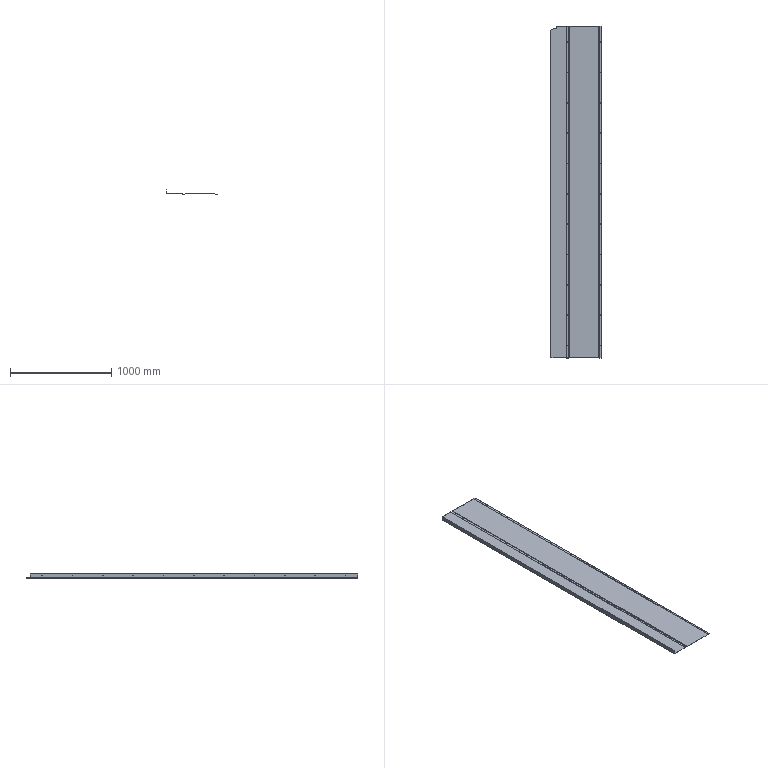Part | STEP file | TS-S100 | 1 solid | 135 faces | box 498 x 3283 x 43 mm | volume 2122569 mm3 | cylinder 83 | plane 52 | commonest cylinder face diameters 5.4 x66 0.4 x7 2.8 x7 10 x1 16 x1 18 x1